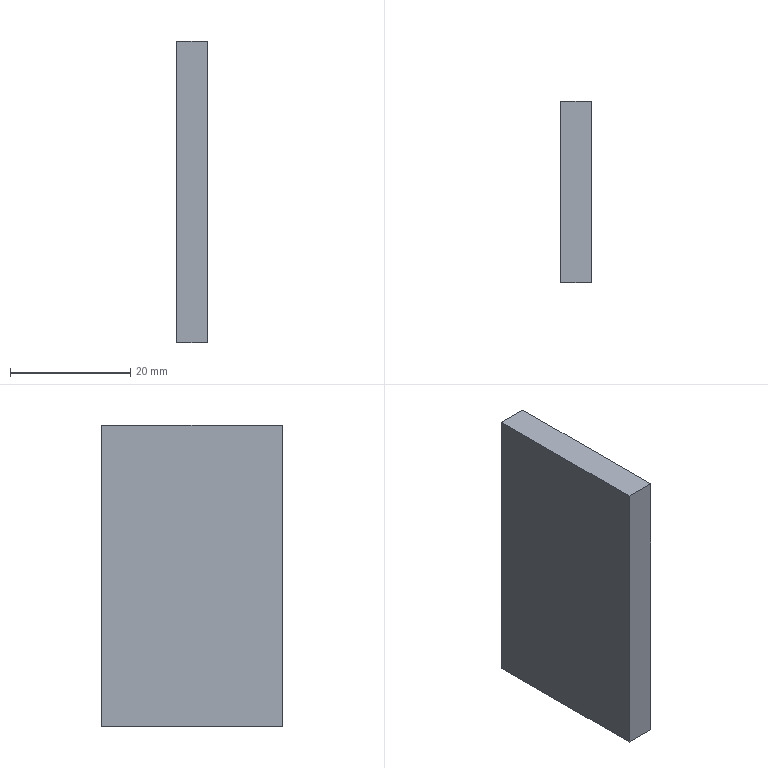Part | SolidWorks | 1 solid | 6 faces | box 5 x 30 x 50 mm | volume 7500 mm3 | plane 6
STEP:
#1=CARTESIAN_POINT('',(0.,15.,25.));
#2=VERTEX_POINT('',#1);
#3=CARTESIAN_POINT('',(0.,-15.,25.));
#4=VERTEX_POINT('',#3);
#5=CARTESIAN_POINT('',(0.,-15.,25.));
#6=DIRECTION('',(0.,-1.,0.));
#7=VECTOR('',#6,1000.);
#8=LINE('',#5,#7);
#9=EDGE_CURVE('',#2,#4,#8,.T.);
#10=ORIENTED_EDGE('',*,*,#9,.F.);
#11=CARTESIAN_POINT('',(-5.,15.,25.));
#12=VERTEX_POINT('',#11);
#13=CARTESIAN_POINT('',(-5.,15.,25.));
#14=DIRECTION('',(1.,0.,0.));
#15=VECTOR('',#14,1000.);
#16=LINE('',#13,#15);
#17=EDGE_CURVE('',#12,#2,#16,.T.);
#18=ORIENTED_EDGE('',*,*,#17,.F.);
#19=CARTESIAN_POINT('',(-5.,-15.,25.));
#20=VERTEX_POINT('',#19);
#21=CARTESIAN_POINT('',(-5.,-15.,25.));
#22=DIRECTION('',(0.,-1.,0.));
#23=VECTOR('',#22,1000.);
#24=LINE('',#21,#23);
#25=EDGE_CURVE('',#12,#20,#24,.T.);
#26=ORIENTED_EDGE('',*,*,#25,.T.);
#27=CARTESIAN_POINT('',(-5.,-15.,25.));
#28=DIRECTION('',(1.,0.,0.));
#29=VECTOR('',#28,1000.);
#30=LINE('',#27,#29);
#31=EDGE_CURVE('',#20,#4,#30,.T.);
#32=ORIENTED_EDGE('',*,*,#31,.T.);
#33=EDGE_LOOP('',(#10,#18,#26,#32));
#34=FACE_OUTER_BOUND('',#33,.T.);
#35=CARTESIAN_POINT('',(-5.,-15.,25.));
#36=DIRECTION('',(0.,0.,1.));
#37=DIRECTION('',(1.,0.,0.));
#38=AXIS2_PLACEMENT_3D('',#35,#36,#37);
#39=PLANE('',#38);
#40=ADVANCED_FACE('',(#34),#39,.T.);
#41=CARTESIAN_POINT('',(0.,15.,-25.));
#42=VERTEX_POINT('',#41);
#43=CARTESIAN_POINT('',(0.,15.,-25.));
#44=DIRECTION('',(0.,0.,1.));
#45=VECTOR('',#44,1000.);
#46=LINE('',#43,#45);
#47=EDGE_CURVE('',#42,#2,#46,.T.);
#48=ORIENTED_EDGE('',*,*,#47,.F.);
#49=CARTESIAN_POINT('',(-5.,15.,-25.));
#50=VERTEX_POINT('',#49);
#51=CARTESIAN_POINT('',(-5.,15.,-25.));
#52=DIRECTION('',(1.,0.,0.));
#53=VECTOR('',#52,1000.);
#54=LINE('',#51,#53);
#55=EDGE_CURVE('',#50,#42,#54,.T.);
#56=ORIENTED_EDGE('',*,*,#55,.F.);
#57=CARTESIAN_POINT('',(-5.,15.,-25.));
#58=DIRECTION('',(0.,0.,1.));
#59=VECTOR('',#58,1000.);
#60=LINE('',#57,#59);
#61=EDGE_CURVE('',#50,#12,#60,.T.);
#62=ORIENTED_EDGE('',*,*,#61,.T.);
#63=ORIENTED_EDGE('',*,*,#17,.T.);
#64=EDGE_LOOP('',(#48,#56,#62,#63));
#65=FACE_OUTER_BOUND('',#64,.T.);
#66=CARTESIAN_POINT('',(-5.,15.,-25.));
#67=DIRECTION('',(0.,1.,0.));
#68=DIRECTION('',(0.,0.,1.));
#69=AXIS2_PLACEMENT_3D('',#66,#67,#68);
#70=PLANE('',#69);
#71=ADVANCED_FACE('',(#65),#70,.T.);
#72=CARTESIAN_POINT('',(0.,-15.,-25.));
#73=VERTEX_POINT('',#72);
#74=CARTESIAN_POINT('',(0.,-15.,-25.));
#75=DIRECTION('',(0.,1.,0.));
#76=VECTOR('',#75,1000.);
#77=LINE('',#74,#76);
#78=EDGE_CURVE('',#73,#42,#77,.T.);
#79=ORIENTED_EDGE('',*,*,#78,.F.);
#80=CARTESIAN_POINT('',(-5.,-15.,-25.));
#81=VERTEX_POINT('',#80);
#82=CARTESIAN_POINT('',(-5.,-15.,-25.));
#83=DIRECTION('',(1.,0.,0.));
#84=VECTOR('',#83,1000.);
#85=LINE('',#82,#84);
#86=EDGE_CURVE('',#81,#73,#85,.T.);
#87=ORIENTED_EDGE('',*,*,#86,.F.);
#88=CARTESIAN_POINT('',(-5.,-15.,-25.));
#89=DIRECTION('',(0.,1.,0.));
#90=VECTOR('',#89,1000.);
#91=LINE('',#88,#90);
#92=EDGE_CURVE('',#81,#50,#91,.T.);
#93=ORIENTED_EDGE('',*,*,#92,.T.);
#94=ORIENTED_EDGE('',*,*,#55,.T.);
#95=EDGE_LOOP('',(#79,#87,#93,#94));
#96=FACE_OUTER_BOUND('',#95,.T.);
#97=CARTESIAN_POINT('',(-5.,-15.,-25.));
#98=DIRECTION('',(0.,0.,-1.));
#99=DIRECTION('',(-1.,0.,0.));
#100=AXIS2_PLACEMENT_3D('',#97,#98,#99);
#101=PLANE('',#100);
#102=ADVANCED_FACE('',(#96),#101,.T.);
#103=CARTESIAN_POINT('',(0.,-15.,-25.));
#104=DIRECTION('',(0.,0.,-1.));
#105=VECTOR('',#104,1000.);
#106=LINE('',#103,#105);
#107=EDGE_CURVE('',#4,#73,#106,.T.);
#108=ORIENTED_EDGE('',*,*,#107,.F.);
#109=ORIENTED_EDGE('',*,*,#31,.F.);
#110=CARTESIAN_POINT('',(-5.,-15.,-25.));
#111=DIRECTION('',(0.,0.,-1.));
#112=VECTOR('',#111,1000.);
#113=LINE('',#110,#112);
#114=EDGE_CURVE('',#20,#81,#113,.T.);
#115=ORIENTED_EDGE('',*,*,#114,.T.);
#116=ORIENTED_EDGE('',*,*,#86,.T.);
#117=EDGE_LOOP('',(#108,#109,#115,#116));
#118=FACE_OUTER_BOUND('',#117,.T.);
#119=CARTESIAN_POINT('',(-5.,-15.,-25.));
#120=DIRECTION('',(0.,-1.,0.));
#121=DIRECTION('',(0.,0.,-1.));
#122=AXIS2_PLACEMENT_3D('',#119,#120,#121);
#123=PLANE('',#122);
#124=ADVANCED_FACE('',(#118),#123,.T.);
#125=ORIENTED_EDGE('',*,*,#25,.F.);
#126=ORIENTED_EDGE('',*,*,#61,.F.);
#127=ORIENTED_EDGE('',*,*,#92,.F.);
#128=ORIENTED_EDGE('',*,*,#114,.F.);
#129=EDGE_LOOP('',(#125,#126,#127,#128));
#130=FACE_OUTER_BOUND('',#129,.T.);
#131=CARTESIAN_POINT('',(-5.,0.,0.));
#132=DIRECTION('',(1.,0.,0.));
#133=DIRECTION('',(0.,0.,-1.));
#134=AXIS2_PLACEMENT_3D('',#131,#132,#133);
#135=PLANE('',#134);
#136=ADVANCED_FACE('',(#130),#135,.F.);
#137=ORIENTED_EDGE('',*,*,#9,.T.);
#138=ORIENTED_EDGE('',*,*,#107,.T.);
#139=ORIENTED_EDGE('',*,*,#78,.T.);
#140=ORIENTED_EDGE('',*,*,#47,.T.);
#141=EDGE_LOOP('',(#137,#138,#139,#140));
#142=FACE_OUTER_BOUND('',#141,.T.);
#143=CARTESIAN_POINT('',(0.,0.,0.));
#144=DIRECTION('',(1.,0.,0.));
#145=DIRECTION('',(0.,0.,-1.));
#146=AXIS2_PLACEMENT_3D('',#143,#144,#145);
#147=PLANE('',#146);
#148=ADVANCED_FACE('',(#142),#147,.T.);
#149=CLOSED_SHELL('',(#40,#71,#102,#124,#136,#148));
#150=MANIFOLD_SOLID_BREP('',#149);
#151=CARTESIAN_POINT('',(0.,0.,0.));
#152=DIRECTION('',(0.,0.,1.));
#153=DIRECTION('',(1.,0.,0.));
#154=AXIS2_PLACEMENT_3D('',#151,#152,#153);
#155=(LENGTH_UNIT()NAMED_UNIT(*)SI_UNIT(.MILLI.,.METRE.));
#156=UNCERTAINTY_MEASURE_WITH_UNIT(LENGTH_MEASURE(0.00001),#155,'','');
#157=(NAMED_UNIT(*)PLANE_ANGLE_UNIT()SI_UNIT($,.RADIAN.));
#158=(NAMED_UNIT(*)SI_UNIT($,.STERADIAN.)SOLID_ANGLE_UNIT());
#159=(GEOMETRIC_REPRESENTATION_CONTEXT(3)GLOBAL_UNCERTAINTY_ASSIGNED_CONTEXT((#156))GLOBAL_UNIT_ASSIGNED_CONTEXT((#155,#157,#158))REPRESENTATION_CONTEXT('',''));
#160=ADVANCED_BREP_SHAPE_REPRESENTATION('',(#150,#154),#159);